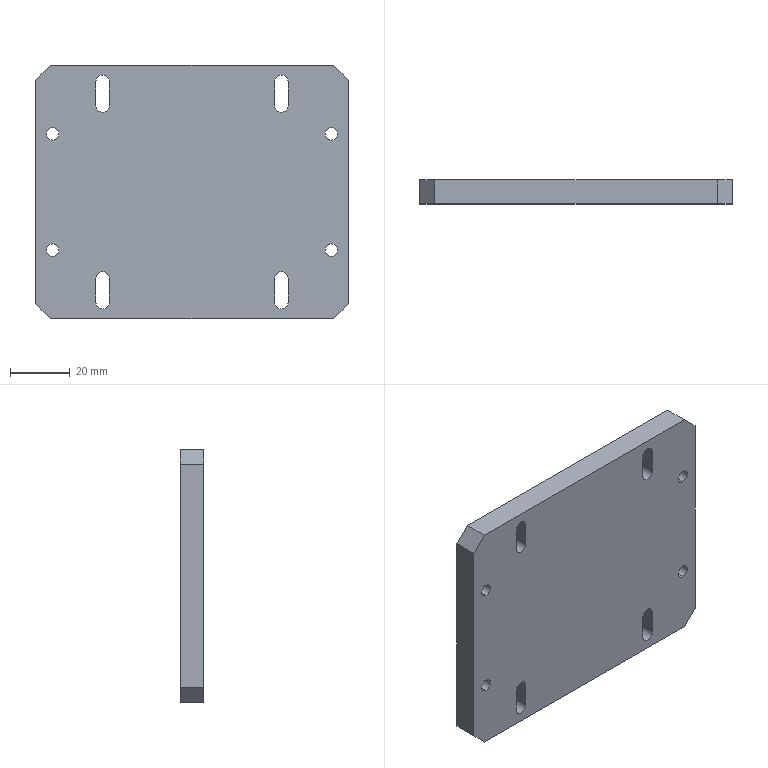Part | STEP file | PN_0023 | 1 solid | 38 faces | box 105 x 8 x 85 mm | volume 68896 mm3 | cylinder 20 | plane 18 | commonest cylinder face diameters 4.5 x12 4.2 x8